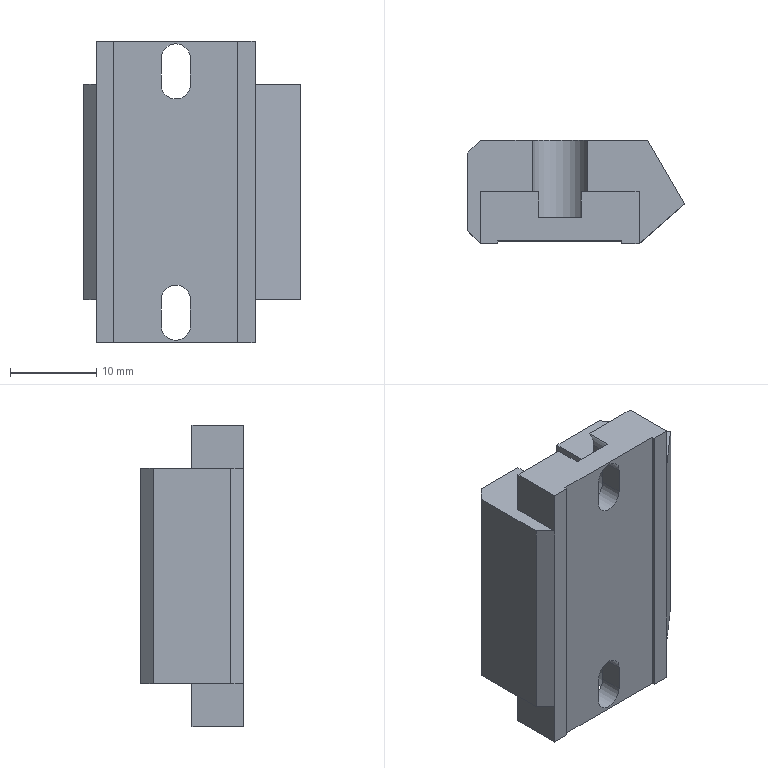Part | SolidWorks | features ICE 10, Chamfer 1, DelFace 1, Extrusion 1, MoveFace 1 | 1 solid | 54 faces | box 25.164 x 12 x 35 mm | volume 7043 mm3 | plane 37 | cylinder 17 | commonest cylinder face diameters 6.4 x7 3.4 x6 4 x4